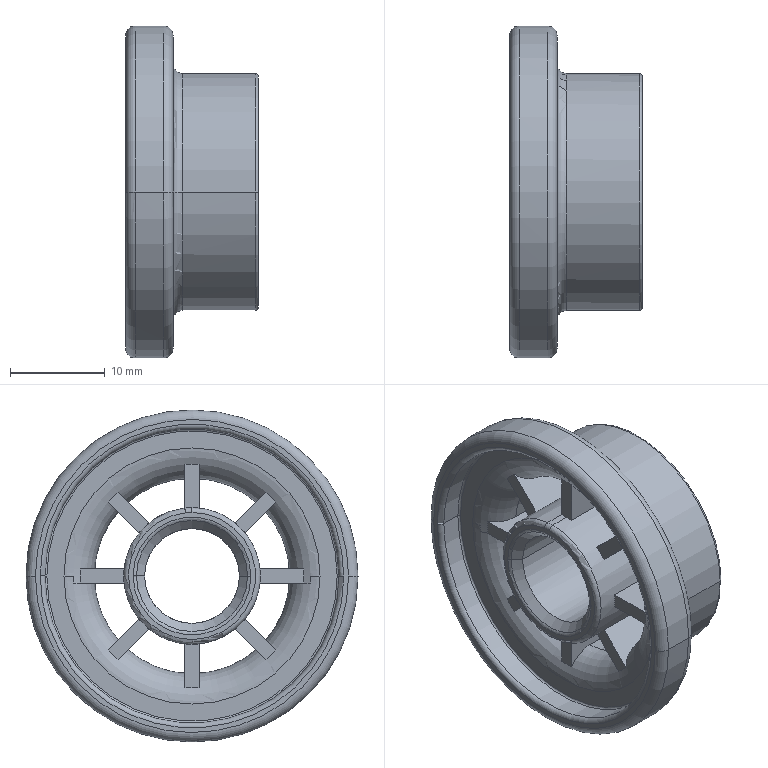Part | STEP file | ZXW735-L-141_2_1_1 | 1 solid | 65 faces | box 14 x 35 x 35 mm | volume 4381 mm3 | plane 31 | torus 18 | cylinder 14 | cone 2 | commonest cylinder face diameters 10 x2 13 x2 14.4 x2 20.6 x2 25 x2 31 x2